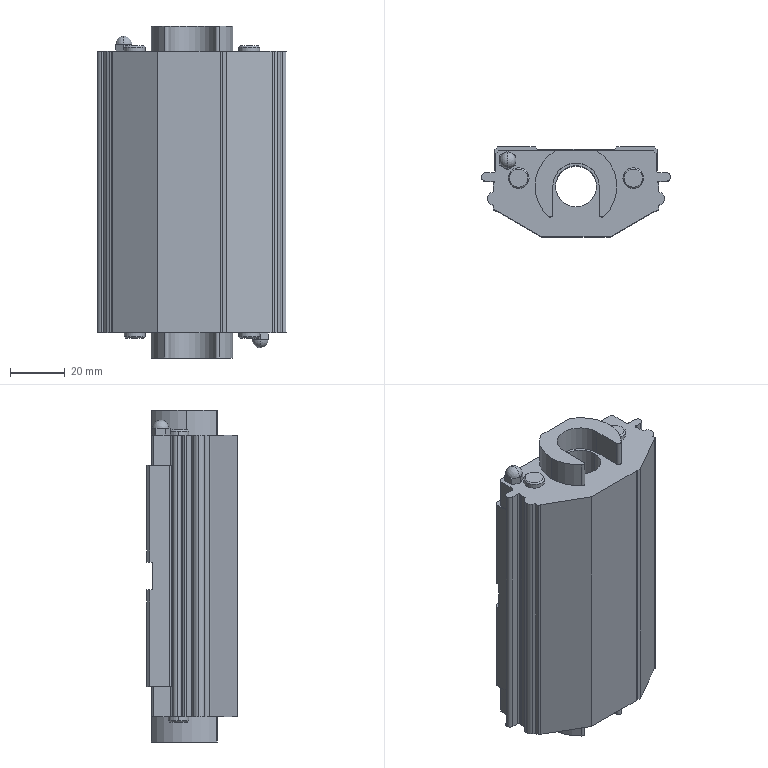Part | STEP file | Guide wheel mechanism revised.sldasm-Part-406 | 1 solid | 191 faces | box 69.2 x 33 x 121.6 mm | volume 172712 mm3 | plane 77 | cone 58 | cylinder 52 | sphere 4 | commonest cylinder face diameters 2 x8 4.917 x8 7.6 x8 30 x6 1.6 x4 2.459 x4